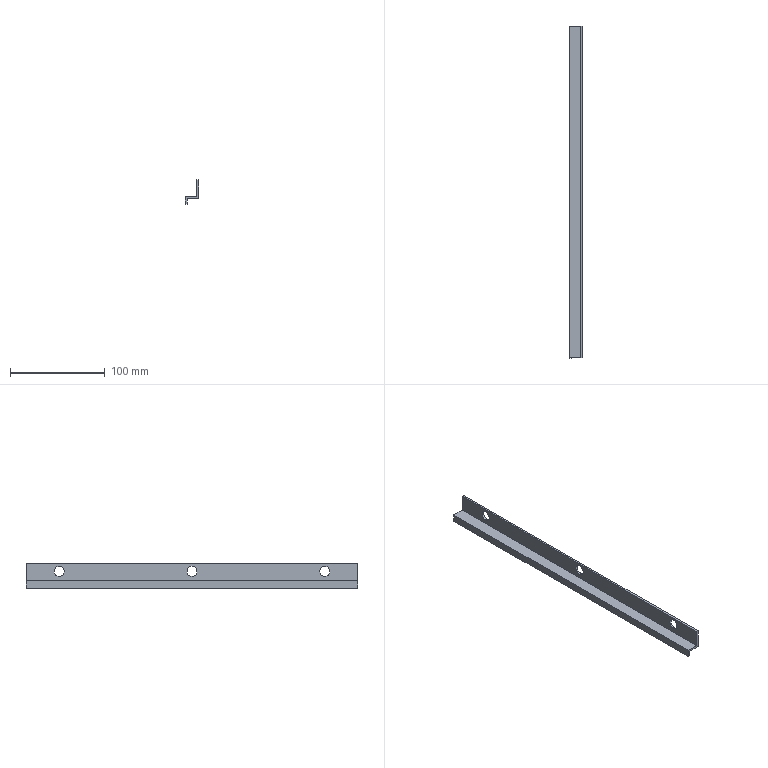Part | SolidWorks | features BaseBody 1 | 1 solid | 16 faces | box 14.5 x 350 x 26 mm | volume 26421 mm3 | plane 10 | cylinder 6 | commonest cylinder face diameters 10.6 x6
STEP:
#1=CARTESIAN_POINT('',(894.946,-4310.973,1968.771));
#2=VERTEX_POINT('',#1);
#3=CARTESIAN_POINT('',(894.946,-4310.973,1958.171));
#4=VERTEX_POINT('',#3);
#5=CARTESIAN_POINT('',(894.946,-4310.973,1963.471));
#6=DIRECTION('',(1.,0.,0.));
#7=DIRECTION('',(0.,0.,-1.));
#8=AXIS2_PLACEMENT_3D('',#5,#6,#7);
#9=CIRCLE('',#8,5.3);
#10=EDGE_CURVE('',#2,#4,#9,.T.);
#11=ORIENTED_EDGE('',*,*,#10,.F.);
#12=CARTESIAN_POINT('',(896.946,-4310.973,1968.771));
#13=VERTEX_POINT('',#12);
#14=CARTESIAN_POINT('',(892.968,-4310.973,1968.771));
#15=DIRECTION('',(1.,0.,0.));
#16=VECTOR('',#15,1000.);
#17=LINE('',#14,#16);
#18=EDGE_CURVE('',#2,#13,#17,.T.);
#19=ORIENTED_EDGE('',*,*,#18,.T.);
#20=CARTESIAN_POINT('',(896.946,-4310.973,1958.171));
#21=VERTEX_POINT('',#20);
#22=CARTESIAN_POINT('',(896.946,-4310.973,1963.471));
#23=DIRECTION('',(-1.,0.,0.));
#24=DIRECTION('',(0.,0.,-1.));
#25=AXIS2_PLACEMENT_3D('',#22,#23,#24);
#26=CIRCLE('',#25,5.3);
#27=EDGE_CURVE('',#21,#13,#26,.T.);
#28=ORIENTED_EDGE('',*,*,#27,.F.);
#29=CARTESIAN_POINT('',(892.968,-4310.973,1958.171));
#30=DIRECTION('',(1.,0.,0.));
#31=VECTOR('',#30,1000.);
#32=LINE('',#29,#31);
#33=EDGE_CURVE('',#4,#21,#32,.T.);
#34=ORIENTED_EDGE('',*,*,#33,.F.);
#35=EDGE_LOOP('',(#11,#19,#28,#34));
#36=FACE_OUTER_BOUND('',#35,.T.);
#37=CARTESIAN_POINT('',(892.968,-4310.973,1963.471));
#38=DIRECTION('',(1.,0.,0.));
#39=DIRECTION('',(0.,0.,-1.));
#40=AXIS2_PLACEMENT_3D('',#37,#38,#39);
#41=CYLINDRICAL_SURFACE('',#40,5.3);
#42=ADVANCED_FACE('',(#36),#41,.F.);
#43=CARTESIAN_POINT('',(894.946,-4030.973,1968.771));
#44=VERTEX_POINT('',#43);
#45=CARTESIAN_POINT('',(894.946,-4030.973,1958.171));
#46=VERTEX_POINT('',#45);
#47=CARTESIAN_POINT('',(894.946,-4030.973,1963.471));
#48=DIRECTION('',(1.,0.,0.));
#49=DIRECTION('',(0.,0.,-1.));
#50=AXIS2_PLACEMENT_3D('',#47,#48,#49);
#51=CIRCLE('',#50,5.3);
#52=EDGE_CURVE('',#44,#46,#51,.T.);
#53=ORIENTED_EDGE('',*,*,#52,.F.);
#54=CARTESIAN_POINT('',(896.946,-4030.973,1968.771));
#55=VERTEX_POINT('',#54);
#56=CARTESIAN_POINT('',(892.968,-4030.973,1968.771));
#57=DIRECTION('',(1.,0.,0.));
#58=VECTOR('',#57,1000.);
#59=LINE('',#56,#58);
#60=EDGE_CURVE('',#44,#55,#59,.T.);
#61=ORIENTED_EDGE('',*,*,#60,.T.);
#62=CARTESIAN_POINT('',(896.946,-4030.973,1958.171));
#63=VERTEX_POINT('',#62);
#64=CARTESIAN_POINT('',(896.946,-4030.973,1963.471));
#65=DIRECTION('',(-1.,0.,0.));
#66=DIRECTION('',(0.,0.,-1.));
#67=AXIS2_PLACEMENT_3D('',#64,#65,#66);
#68=CIRCLE('',#67,5.3);
#69=EDGE_CURVE('',#63,#55,#68,.T.);
#70=ORIENTED_EDGE('',*,*,#69,.F.);
#71=CARTESIAN_POINT('',(892.968,-4030.973,1958.171));
#72=DIRECTION('',(1.,0.,0.));
#73=VECTOR('',#72,1000.);
#74=LINE('',#71,#73);
#75=EDGE_CURVE('',#46,#63,#74,.T.);
#76=ORIENTED_EDGE('',*,*,#75,.F.);
#77=EDGE_LOOP('',(#53,#61,#70,#76));
#78=FACE_OUTER_BOUND('',#77,.T.);
#79=CARTESIAN_POINT('',(892.968,-4030.973,1963.471));
#80=DIRECTION('',(1.,0.,0.));
#81=DIRECTION('',(0.,0.,-1.));
#82=AXIS2_PLACEMENT_3D('',#79,#80,#81);
#83=CYLINDRICAL_SURFACE('',#82,5.3);
#84=ADVANCED_FACE('',(#78),#83,.F.);
#85=CARTESIAN_POINT('',(894.946,-4170.973,1968.771));
#86=VERTEX_POINT('',#85);
#87=CARTESIAN_POINT('',(894.946,-4170.973,1958.171));
#88=VERTEX_POINT('',#87);
#89=CARTESIAN_POINT('',(894.946,-4170.973,1963.471));
#90=DIRECTION('',(1.,0.,0.));
#91=DIRECTION('',(0.,0.,-1.));
#92=AXIS2_PLACEMENT_3D('',#89,#90,#91);
#93=CIRCLE('',#92,5.3);
#94=EDGE_CURVE('',#86,#88,#93,.T.);
#95=ORIENTED_EDGE('',*,*,#94,.F.);
#96=CARTESIAN_POINT('',(896.946,-4170.973,1968.771));
#97=VERTEX_POINT('',#96);
#98=CARTESIAN_POINT('',(892.968,-4170.973,1968.771));
#99=DIRECTION('',(1.,0.,0.));
#100=VECTOR('',#99,1000.);
#101=LINE('',#98,#100);
#102=EDGE_CURVE('',#86,#97,#101,.T.);
#103=ORIENTED_EDGE('',*,*,#102,.T.);
#104=CARTESIAN_POINT('',(896.946,-4170.973,1958.171));
#105=VERTEX_POINT('',#104);
#106=CARTESIAN_POINT('',(896.946,-4170.973,1963.471));
#107=DIRECTION('',(-1.,0.,0.));
#108=DIRECTION('',(0.,0.,-1.));
#109=AXIS2_PLACEMENT_3D('',#106,#107,#108);
#110=CIRCLE('',#109,5.3);
#111=EDGE_CURVE('',#105,#97,#110,.T.);
#112=ORIENTED_EDGE('',*,*,#111,.F.);
#113=CARTESIAN_POINT('',(892.968,-4170.973,1958.171));
#114=DIRECTION('',(1.,0.,0.));
#115=VECTOR('',#114,1000.);
#116=LINE('',#113,#115);
#117=EDGE_CURVE('',#88,#105,#116,.T.);
#118=ORIENTED_EDGE('',*,*,#117,.F.);
#119=EDGE_LOOP('',(#95,#103,#112,#118));
#120=FACE_OUTER_BOUND('',#119,.T.);
#121=CARTESIAN_POINT('',(892.968,-4170.973,1963.471));
#122=DIRECTION('',(1.,0.,0.));
#123=DIRECTION('',(0.,0.,-1.));
#124=AXIS2_PLACEMENT_3D('',#121,#122,#123);
#125=CYLINDRICAL_SURFACE('',#124,5.3);
#126=ADVANCED_FACE('',(#120),#125,.F.);
#127=CARTESIAN_POINT('',(896.946,-3995.973,1951.471));
#128=VERTEX_POINT('',#127);
#129=CARTESIAN_POINT('',(896.946,-3995.973,1971.471));
#130=VERTEX_POINT('',#129);
#131=CARTESIAN_POINT('',(896.946,-3995.973,1951.471));
#132=DIRECTION('',(0.,0.,1.));
#133=VECTOR('',#132,1000.);
#134=LINE('',#131,#133);
#135=EDGE_CURVE('',#128,#130,#134,.T.);
#136=ORIENTED_EDGE('',*,*,#135,.T.);
#137=CARTESIAN_POINT('',(896.946,-4345.973,1971.471));
#138=VERTEX_POINT('',#137);
#139=CARTESIAN_POINT('',(896.946,-3995.973,1971.471));
#140=DIRECTION('',(0.,-1.,0.));
#141=VECTOR('',#140,1000.);
#142=LINE('',#139,#141);
#143=EDGE_CURVE('',#130,#138,#142,.T.);
#144=ORIENTED_EDGE('',*,*,#143,.T.);
#145=CARTESIAN_POINT('',(896.946,-4345.973,1951.471));
#146=VERTEX_POINT('',#145);
#147=CARTESIAN_POINT('',(896.946,-4345.973,1951.471));
#148=DIRECTION('',(0.,0.,-1.));
#149=VECTOR('',#148,1000.);
#150=LINE('',#147,#149);
#151=EDGE_CURVE('',#138,#146,#150,.T.);
#152=ORIENTED_EDGE('',*,*,#151,.T.);
#153=CARTESIAN_POINT('',(896.946,-3995.973,1951.471));
#154=DIRECTION('',(0.,1.,0.));
#155=VECTOR('',#154,1000.);
#156=LINE('',#153,#155);
#157=EDGE_CURVE('',#146,#128,#156,.T.);
#158=ORIENTED_EDGE('',*,*,#157,.T.);
#159=EDGE_LOOP('',(#136,#144,#152,#158));
#160=FACE_OUTER_BOUND('',#159,.T.);
#161=ORIENTED_EDGE('',*,*,#27,.T.);
#162=CARTESIAN_POINT('',(896.946,-4310.973,1963.471));
#163=DIRECTION('',(-1.,0.,0.));
#164=DIRECTION('',(0.,0.,-1.));
#165=AXIS2_PLACEMENT_3D('',#162,#163,#164);
#166=CIRCLE('',#165,5.3);
#167=EDGE_CURVE('',#13,#21,#166,.T.);
#168=ORIENTED_EDGE('',*,*,#167,.T.);
#169=EDGE_LOOP('',(#161,#168));
#170=FACE_BOUND('',#169,.T.);
#171=ORIENTED_EDGE('',*,*,#69,.T.);
#172=CARTESIAN_POINT('',(896.946,-4030.973,1963.471));
#173=DIRECTION('',(-1.,0.,0.));
#174=DIRECTION('',(0.,0.,-1.));
#175=AXIS2_PLACEMENT_3D('',#172,#173,#174);
#176=CIRCLE('',#175,5.3);
#177=EDGE_CURVE('',#55,#63,#176,.T.);
#178=ORIENTED_EDGE('',*,*,#177,.T.);
#179=EDGE_LOOP('',(#171,#178));
#180=FACE_BOUND('',#179,.T.);
#181=ORIENTED_EDGE('',*,*,#111,.T.);
#182=CARTESIAN_POINT('',(896.946,-4170.973,1963.471));
#183=DIRECTION('',(-1.,0.,0.));
#184=DIRECTION('',(0.,0.,-1.));
#185=AXIS2_PLACEMENT_3D('',#182,#183,#184);
#186=CIRCLE('',#185,5.3);
#187=EDGE_CURVE('',#97,#105,#186,.T.);
#188=ORIENTED_EDGE('',*,*,#187,.T.);
#189=EDGE_LOOP('',(#181,#188));
#190=FACE_BOUND('',#189,.T.);
#191=CARTESIAN_POINT('',(896.946,-3995.973,1951.471));
#192=DIRECTION('',(1.,0.,0.));
#193=DIRECTION('',(0.,0.,-1.));
#194=AXIS2_PLACEMENT_3D('',#191,#192,#193);
#195=PLANE('',#194);
#196=ADVANCED_FACE('',(#160,#170,#180,#190),#195,.T.);
#197=CARTESIAN_POINT('',(894.946,-3995.973,1971.471));
#198=VERTEX_POINT('',#197);
#199=CARTESIAN_POINT('',(896.946,-3995.973,1971.471));
#200=DIRECTION('',(-1.,0.,0.));
#201=VECTOR('',#200,1000.);
#202=LINE('',#199,#201);
#203=EDGE_CURVE('',#130,#198,#202,.T.);
#204=ORIENTED_EDGE('',*,*,#203,.T.);
#205=CARTESIAN_POINT('',(894.946,-4345.973,1971.471));
#206=VERTEX_POINT('',#205);
#207=CARTESIAN_POINT('',(894.946,-3995.973,1971.471));
#208=DIRECTION('',(0.,-1.,0.));
#209=VECTOR('',#208,1000.);
#210=LINE('',#207,#209);
#211=EDGE_CURVE('',#198,#206,#210,.T.);
#212=ORIENTED_EDGE('',*,*,#211,.T.);
#213=CARTESIAN_POINT('',(896.946,-4345.973,1971.471));
#214=DIRECTION('',(1.,0.,0.));
#215=VECTOR('',#214,1000.);
#216=LINE('',#213,#215);
#217=EDGE_CURVE('',#206,#138,#216,.T.);
#218=ORIENTED_EDGE('',*,*,#217,.T.);
#219=ORIENTED_EDGE('',*,*,#143,.F.);
#220=EDGE_LOOP('',(#204,#212,#218,#219));
#221=FACE_OUTER_BOUND('',#220,.T.);
#222=CARTESIAN_POINT('',(896.946,-3995.973,1971.471));
#223=DIRECTION('',(0.,0.,1.));
#224=DIRECTION('',(1.,0.,0.));
#225=AXIS2_PLACEMENT_3D('',#222,#223,#224);
#226=PLANE('',#225);
#227=ADVANCED_FACE('',(#221),#226,.T.);
#228=CARTESIAN_POINT('',(882.446,-3995.973,1945.471));
#229=VERTEX_POINT('',#228);
#230=CARTESIAN_POINT('',(882.446,-3995.973,1953.471));
#231=VERTEX_POINT('',#230);
#232=CARTESIAN_POINT('',(882.446,-3995.973,1956.835));
#233=DIRECTION('',(0.,0.,1.));
#234=VECTOR('',#233,1000.);
#235=LINE('',#232,#234);
#236=EDGE_CURVE('',#229,#231,#235,.T.);
#237=ORIENTED_EDGE('',*,*,#236,.T.);
#238=CARTESIAN_POINT('',(894.946,-3995.973,1953.471));
#239=VERTEX_POINT('',#238);
#240=CARTESIAN_POINT('',(892.332,-3995.973,1953.471));
#241=DIRECTION('',(1.,0.,0.));
#242=VECTOR('',#241,1000.);
#243=LINE('',#240,#242);
#244=EDGE_CURVE('',#231,#239,#243,.T.);
#245=ORIENTED_EDGE('',*,*,#244,.T.);
#246=CARTESIAN_POINT('',(894.946,-3995.973,1956.835));
#247=DIRECTION('',(0.,0.,1.));
#248=VECTOR('',#247,1000.);
#249=LINE('',#246,#248);
#250=EDGE_CURVE('',#239,#198,#249,.T.);
#251=ORIENTED_EDGE('',*,*,#250,.T.);
#252=ORIENTED_EDGE('',*,*,#203,.F.);
#253=ORIENTED_EDGE('',*,*,#135,.F.);
#254=CARTESIAN_POINT('',(884.446,-3995.973,1951.471));
#255=VERTEX_POINT('',#254);
#256=CARTESIAN_POINT('',(892.332,-3995.973,1951.471));
#257=DIRECTION('',(-1.,0.,0.));
#258=VECTOR('',#257,1000.);
#259=LINE('',#256,#258);
#260=EDGE_CURVE('',#128,#255,#259,.T.);
#261=ORIENTED_EDGE('',*,*,#260,.T.);
#262=CARTESIAN_POINT('',(884.446,-3995.973,1945.471));
#263=VERTEX_POINT('',#262);
#264=CARTESIAN_POINT('',(884.446,-3995.973,1956.835));
#265=DIRECTION('',(0.,0.,-1.));
#266=VECTOR('',#265,1000.);
#267=LINE('',#264,#266);
#268=EDGE_CURVE('',#255,#263,#267,.T.);
#269=ORIENTED_EDGE('',*,*,#268,.T.);
#270=CARTESIAN_POINT('',(892.332,-3995.973,1945.471));
#271=DIRECTION('',(-1.,0.,0.));
#272=VECTOR('',#271,1000.);
#273=LINE('',#270,#272);
#274=EDGE_CURVE('',#263,#229,#273,.T.);
#275=ORIENTED_EDGE('',*,*,#274,.T.);
#276=EDGE_LOOP('',(#237,#245,#251,#252,#253,#261,#269,#275));
#277=FACE_OUTER_BOUND('',#276,.T.);
#278=CARTESIAN_POINT('',(892.332,-3995.973,1956.835));
#279=DIRECTION('',(0.,1.,0.));
#280=DIRECTION('',(0.,0.,1.));
#281=AXIS2_PLACEMENT_3D('',#278,#279,#280);
#282=PLANE('',#281);
#283=ADVANCED_FACE('',(#277),#282,.T.);
#284=ORIENTED_EDGE('',*,*,#260,.F.);
#285=ORIENTED_EDGE('',*,*,#157,.F.);
#286=CARTESIAN_POINT('',(884.446,-4345.973,1951.471));
#287=VERTEX_POINT('',#286);
#288=CARTESIAN_POINT('',(886.446,-4345.973,1951.471));
#289=DIRECTION('',(-1.,0.,0.));
#290=VECTOR('',#289,1000.);
#291=LINE('',#288,#290);
#292=EDGE_CURVE('',#146,#287,#291,.T.);
#293=ORIENTED_EDGE('',*,*,#292,.T.);
#294=CARTESIAN_POINT('',(884.446,-3995.973,1951.471));
#295=DIRECTION('',(0.,1.,0.));
#296=VECTOR('',#295,1000.);
#297=LINE('',#294,#296);
#298=EDGE_CURVE('',#287,#255,#297,.T.);
#299=ORIENTED_EDGE('',*,*,#298,.T.);
#300=EDGE_LOOP('',(#284,#285,#293,#299));
#301=FACE_OUTER_BOUND('',#300,.T.);
#302=CARTESIAN_POINT('',(886.446,-3995.973,1951.471));
#303=DIRECTION('',(0.,0.,-1.));
#304=DIRECTION('',(-1.,0.,0.));
#305=AXIS2_PLACEMENT_3D('',#302,#303,#304);
#306=PLANE('',#305);
#307=ADVANCED_FACE('',(#301),#306,.T.);
#308=CARTESIAN_POINT('',(882.446,-4345.973,1945.471));
#309=VERTEX_POINT('',#308);
#310=CARTESIAN_POINT('',(882.446,-4345.973,1953.471));
#311=VERTEX_POINT('',#310);
#312=CARTESIAN_POINT('',(882.446,-4345.973,1956.835));
#313=DIRECTION('',(0.,0.,1.));
#314=VECTOR('',#313,1000.);
#315=LINE('',#312,#314);
#316=EDGE_CURVE('',#309,#311,#315,.T.);
#317=ORIENTED_EDGE('',*,*,#316,.F.);
#318=CARTESIAN_POINT('',(884.446,-4345.973,1945.471));
#319=VERTEX_POINT('',#318);
#320=CARTESIAN_POINT('',(890.832,-4345.973,1945.471));
#321=DIRECTION('',(-1.,0.,0.));
#322=VECTOR('',#321,1000.);
#323=LINE('',#320,#322);
#324=EDGE_CURVE('',#319,#309,#323,.T.);
#325=ORIENTED_EDGE('',*,*,#324,.F.);
#326=CARTESIAN_POINT('',(884.446,-4345.973,1956.835));
#327=DIRECTION('',(0.,0.,-1.));
#328=VECTOR('',#327,1000.);
#329=LINE('',#326,#328);
#330=EDGE_CURVE('',#287,#319,#329,.T.);
#331=ORIENTED_EDGE('',*,*,#330,.F.);
#332=ORIENTED_EDGE('',*,*,#292,.F.);
#333=ORIENTED_EDGE('',*,*,#151,.F.);
#334=ORIENTED_EDGE('',*,*,#217,.F.);
#335=CARTESIAN_POINT('',(894.946,-4345.973,1953.471));
#336=VERTEX_POINT('',#335);
#337=CARTESIAN_POINT('',(894.946,-4345.973,1956.835));
#338=DIRECTION('',(0.,0.,1.));
#339=VECTOR('',#338,1000.);
#340=LINE('',#337,#339);
#341=EDGE_CURVE('',#336,#206,#340,.T.);
#342=ORIENTED_EDGE('',*,*,#341,.F.);
#343=CARTESIAN_POINT('',(890.832,-4345.973,1953.471));
#344=DIRECTION('',(1.,0.,0.));
#345=VECTOR('',#344,1000.);
#346=LINE('',#343,#345);
#347=EDGE_CURVE('',#311,#336,#346,.T.);
#348=ORIENTED_EDGE('',*,*,#347,.F.);
#349=EDGE_LOOP('',(#317,#325,#331,#332,#333,#334,#342,#348));
#350=FACE_OUTER_BOUND('',#349,.T.);
#351=CARTESIAN_POINT('',(890.832,-4345.973,1956.835));
#352=DIRECTION('',(0.,1.,0.));
#353=DIRECTION('',(0.,0.,1.));
#354=AXIS2_PLACEMENT_3D('',#351,#352,#353);
#355=PLANE('',#354);
#356=ADVANCED_FACE('',(#350),#355,.F.);
#357=ORIENTED_EDGE('',*,*,#18,.F.);
#358=CARTESIAN_POINT('',(894.946,-4310.973,1963.471));
#359=DIRECTION('',(1.,0.,0.));
#360=DIRECTION('',(0.,0.,-1.));
#361=AXIS2_PLACEMENT_3D('',#358,#359,#360);
#362=CIRCLE('',#361,5.3);
#363=EDGE_CURVE('',#4,#2,#362,.T.);
#364=ORIENTED_EDGE('',*,*,#363,.F.);
#365=ORIENTED_EDGE('',*,*,#33,.T.);
#366=ORIENTED_EDGE('',*,*,#167,.F.);
#367=EDGE_LOOP('',(#357,#364,#365,#366));
#368=FACE_OUTER_BOUND('',#367,.T.);
#369=CARTESIAN_POINT('',(892.968,-4310.973,1963.471));
#370=DIRECTION('',(1.,0.,0.));
#371=DIRECTION('',(0.,0.,-1.));
#372=AXIS2_PLACEMENT_3D('',#369,#370,#371);
#373=CYLINDRICAL_SURFACE('',#372,5.3);
#374=ADVANCED_FACE('',(#368),#373,.F.);
#375=ORIENTED_EDGE('',*,*,#60,.F.);
#376=CARTESIAN_POINT('',(894.946,-4030.973,1963.471));
#377=DIRECTION('',(1.,0.,0.));
#378=DIRECTION('',(0.,0.,-1.));
#379=AXIS2_PLACEMENT_3D('',#376,#377,#378);
#380=CIRCLE('',#379,5.3);
#381=EDGE_CURVE('',#46,#44,#380,.T.);
#382=ORIENTED_EDGE('',*,*,#381,.F.);
#383=ORIENTED_EDGE('',*,*,#75,.T.);
#384=ORIENTED_EDGE('',*,*,#177,.F.);
#385=EDGE_LOOP('',(#375,#382,#383,#384));
#386=FACE_OUTER_BOUND('',#385,.T.);
#387=CARTESIAN_POINT('',(892.968,-4030.973,1963.471));
#388=DIRECTION('',(1.,0.,0.));
#389=DIRECTION('',(0.,0.,-1.));
#390=AXIS2_PLACEMENT_3D('',#387,#388,#389);
#391=CYLINDRICAL_SURFACE('',#390,5.3);
#392=ADVANCED_FACE('',(#386),#391,.F.);
#393=ORIENTED_EDGE('',*,*,#102,.F.);
#394=CARTESIAN_POINT('',(894.946,-4170.973,1963.471));
#395=DIRECTION('',(1.,0.,0.));
#396=DIRECTION('',(0.,0.,-1.));
#397=AXIS2_PLACEMENT_3D('',#394,#395,#396);
#398=CIRCLE('',#397,5.3);
#399=EDGE_CURVE('',#88,#86,#398,.T.);
#400=ORIENTED_EDGE('',*,*,#399,.F.);
#401=ORIENTED_EDGE('',*,*,#117,.T.);
#402=ORIENTED_EDGE('',*,*,#187,.F.);
#403=EDGE_LOOP('',(#393,#400,#401,#402));
#404=FACE_OUTER_BOUND('',#403,.T.);
#405=CARTESIAN_POINT('',(892.968,-4170.973,1963.471));
#406=DIRECTION('',(1.,0.,0.));
#407=DIRECTION('',(0.,0.,-1.));
#408=AXIS2_PLACEMENT_3D('',#405,#406,#407);
#409=CYLINDRICAL_SURFACE('',#408,5.3);
#410=ADVANCED_FACE('',(#404),#409,.F.);
#411=ORIENTED_EDGE('',*,*,#250,.F.);
#412=CARTESIAN_POINT('',(894.946,-3995.973,1953.471));
#413=DIRECTION('',(0.,-1.,0.));
#414=VECTOR('',#413,1000.);
#415=LINE('',#412,#414);
#416=EDGE_CURVE('',#239,#336,#415,.T.);
#417=ORIENTED_EDGE('',*,*,#416,.T.);
#418=ORIENTED_EDGE('',*,*,#341,.T.);
#419=ORIENTED_EDGE('',*,*,#211,.F.);
#420=EDGE_LOOP('',(#411,#417,#418,#419));
#421=FACE_OUTER_BOUND('',#420,.T.);
#422=ORIENTED_EDGE('',*,*,#363,.T.);
#423=ORIENTED_EDGE('',*,*,#10,.T.);
#424=EDGE_LOOP('',(#422,#423));
#425=FACE_BOUND('',#424,.T.);
#426=ORIENTED_EDGE('',*,*,#381,.T.);
#427=ORIENTED_EDGE('',*,*,#52,.T.);
#428=EDGE_LOOP('',(#426,#427));
#429=FACE_BOUND('',#428,.T.);
#430=ORIENTED_EDGE('',*,*,#399,.T.);
#431=ORIENTED_EDGE('',*,*,#94,.T.);
#432=EDGE_LOOP('',(#430,#431));
#433=FACE_BOUND('',#432,.T.);
#434=CARTESIAN_POINT('',(894.946,-3995.973,1971.471));
#435=DIRECTION('',(-1.,0.,0.));
#436=DIRECTION('',(0.,0.,1.));
#437=AXIS2_PLACEMENT_3D('',#434,#435,#436);
#438=PLANE('',#437);
#439=ADVANCED_FACE('',(#421,#425,#429,#433),#438,.T.);
#440=ORIENTED_EDGE('',*,*,#244,.F.);
#441=CARTESIAN_POINT('',(882.446,-3995.973,1953.471));
#442=DIRECTION('',(0.,-1.,0.));
#443=VECTOR('',#442,1000.);
#444=LINE('',#441,#443);
#445=EDGE_CURVE('',#231,#311,#444,.T.);
#446=ORIENTED_EDGE('',*,*,#445,.T.);
#447=ORIENTED_EDGE('',*,*,#347,.T.);
#448=ORIENTED_EDGE('',*,*,#416,.F.);
#449=EDGE_LOOP('',(#440,#446,#447,#448));
#450=FACE_OUTER_BOUND('',#449,.T.);
#451=CARTESIAN_POINT('',(892.446,-3995.973,1953.471));
#452=DIRECTION('',(0.,0.,1.));
#453=DIRECTION('',(1.,0.,0.));
#454=AXIS2_PLACEMENT_3D('',#451,#452,#453);
#455=PLANE('',#454);
#456=ADVANCED_FACE('',(#450),#455,.T.);
#457=ORIENTED_EDGE('',*,*,#236,.F.);
#458=CARTESIAN_POINT('',(882.446,-3995.973,1945.471));
#459=DIRECTION('',(0.,-1.,0.));
#460=VECTOR('',#459,1000.);
#461=LINE('',#458,#460);
#462=EDGE_CURVE('',#229,#309,#461,.T.);
#463=ORIENTED_EDGE('',*,*,#462,.T.);
#464=ORIENTED_EDGE('',*,*,#316,.T.);
#465=ORIENTED_EDGE('',*,*,#445,.F.);
#466=EDGE_LOOP('',(#457,#463,#464,#465));
#467=FACE_OUTER_BOUND('',#466,.T.);
#468=CARTESIAN_POINT('',(882.446,-3995.973,1953.471));
#469=DIRECTION('',(-1.,0.,0.));
#470=DIRECTION('',(0.,0.,1.));
#471=AXIS2_PLACEMENT_3D('',#468,#469,#470);
#472=PLANE('',#471);
#473=ADVANCED_FACE('',(#467),#472,.T.);
#474=ORIENTED_EDGE('',*,*,#274,.F.);
#475=CARTESIAN_POINT('',(884.446,-3995.973,1945.471));
#476=DIRECTION('',(0.,-1.,0.));
#477=VECTOR('',#476,1000.);
#478=LINE('',#475,#477);
#479=EDGE_CURVE('',#263,#319,#478,.T.);
#480=ORIENTED_EDGE('',*,*,#479,.T.);
#481=ORIENTED_EDGE('',*,*,#324,.T.);
#482=ORIENTED_EDGE('',*,*,#462,.F.);
#483=EDGE_LOOP('',(#474,#480,#481,#482));
#484=FACE_OUTER_BOUND('',#483,.T.);
#485=CARTESIAN_POINT('',(884.446,-3995.973,1945.471));
#486=DIRECTION('',(0.,0.,-1.));
#487=DIRECTION('',(-1.,0.,0.));
#488=AXIS2_PLACEMENT_3D('',#485,#486,#487);
#489=PLANE('',#488);
#490=ADVANCED_FACE('',(#484),#489,.T.);
#491=ORIENTED_EDGE('',*,*,#268,.F.);
#492=ORIENTED_EDGE('',*,*,#298,.F.);
#493=ORIENTED_EDGE('',*,*,#330,.T.);
#494=ORIENTED_EDGE('',*,*,#479,.F.);
#495=EDGE_LOOP('',(#491,#492,#493,#494));
#496=FACE_OUTER_BOUND('',#495,.T.);
#497=CARTESIAN_POINT('',(884.446,-3995.973,1945.471));
#498=DIRECTION('',(1.,0.,0.));
#499=DIRECTION('',(0.,0.,-1.));
#500=AXIS2_PLACEMENT_3D('',#497,#498,#499);
#501=PLANE('',#500);
#502=ADVANCED_FACE('',(#496),#501,.T.);
#503=CLOSED_SHELL('',(#42,#84,#126,#196,#227,#283,#307,#356,#374,#392,#410,#439,#456,#473,#490,#502));
#504=MANIFOLD_SOLID_BREP('',#503);
#505=CARTESIAN_POINT('',(0.,0.,0.));
#506=DIRECTION('',(0.,0.,1.));
#507=DIRECTION('',(1.,0.,0.));
#508=AXIS2_PLACEMENT_3D('',#505,#506,#507);
#509=(LENGTH_UNIT()NAMED_UNIT(*)SI_UNIT(.MILLI.,.METRE.));
#510=UNCERTAINTY_MEASURE_WITH_UNIT(LENGTH_MEASURE(0.00001),#509,'','');
#511=(NAMED_UNIT(*)PLANE_ANGLE_UNIT()SI_UNIT($,.RADIAN.));
#512=(NAMED_UNIT(*)SI_UNIT($,.STERADIAN.)SOLID_ANGLE_UNIT());
#513=(GEOMETRIC_REPRESENTATION_CONTEXT(3)GLOBAL_UNCERTAINTY_ASSIGNED_CONTEXT((#510))GLOBAL_UNIT_ASSIGNED_CONTEXT((#509,#511,#512))REPRESENTATION_CONTEXT('',''));
#514=ADVANCED_BREP_SHAPE_REPRESENTATION('',(#504,#508),#513);